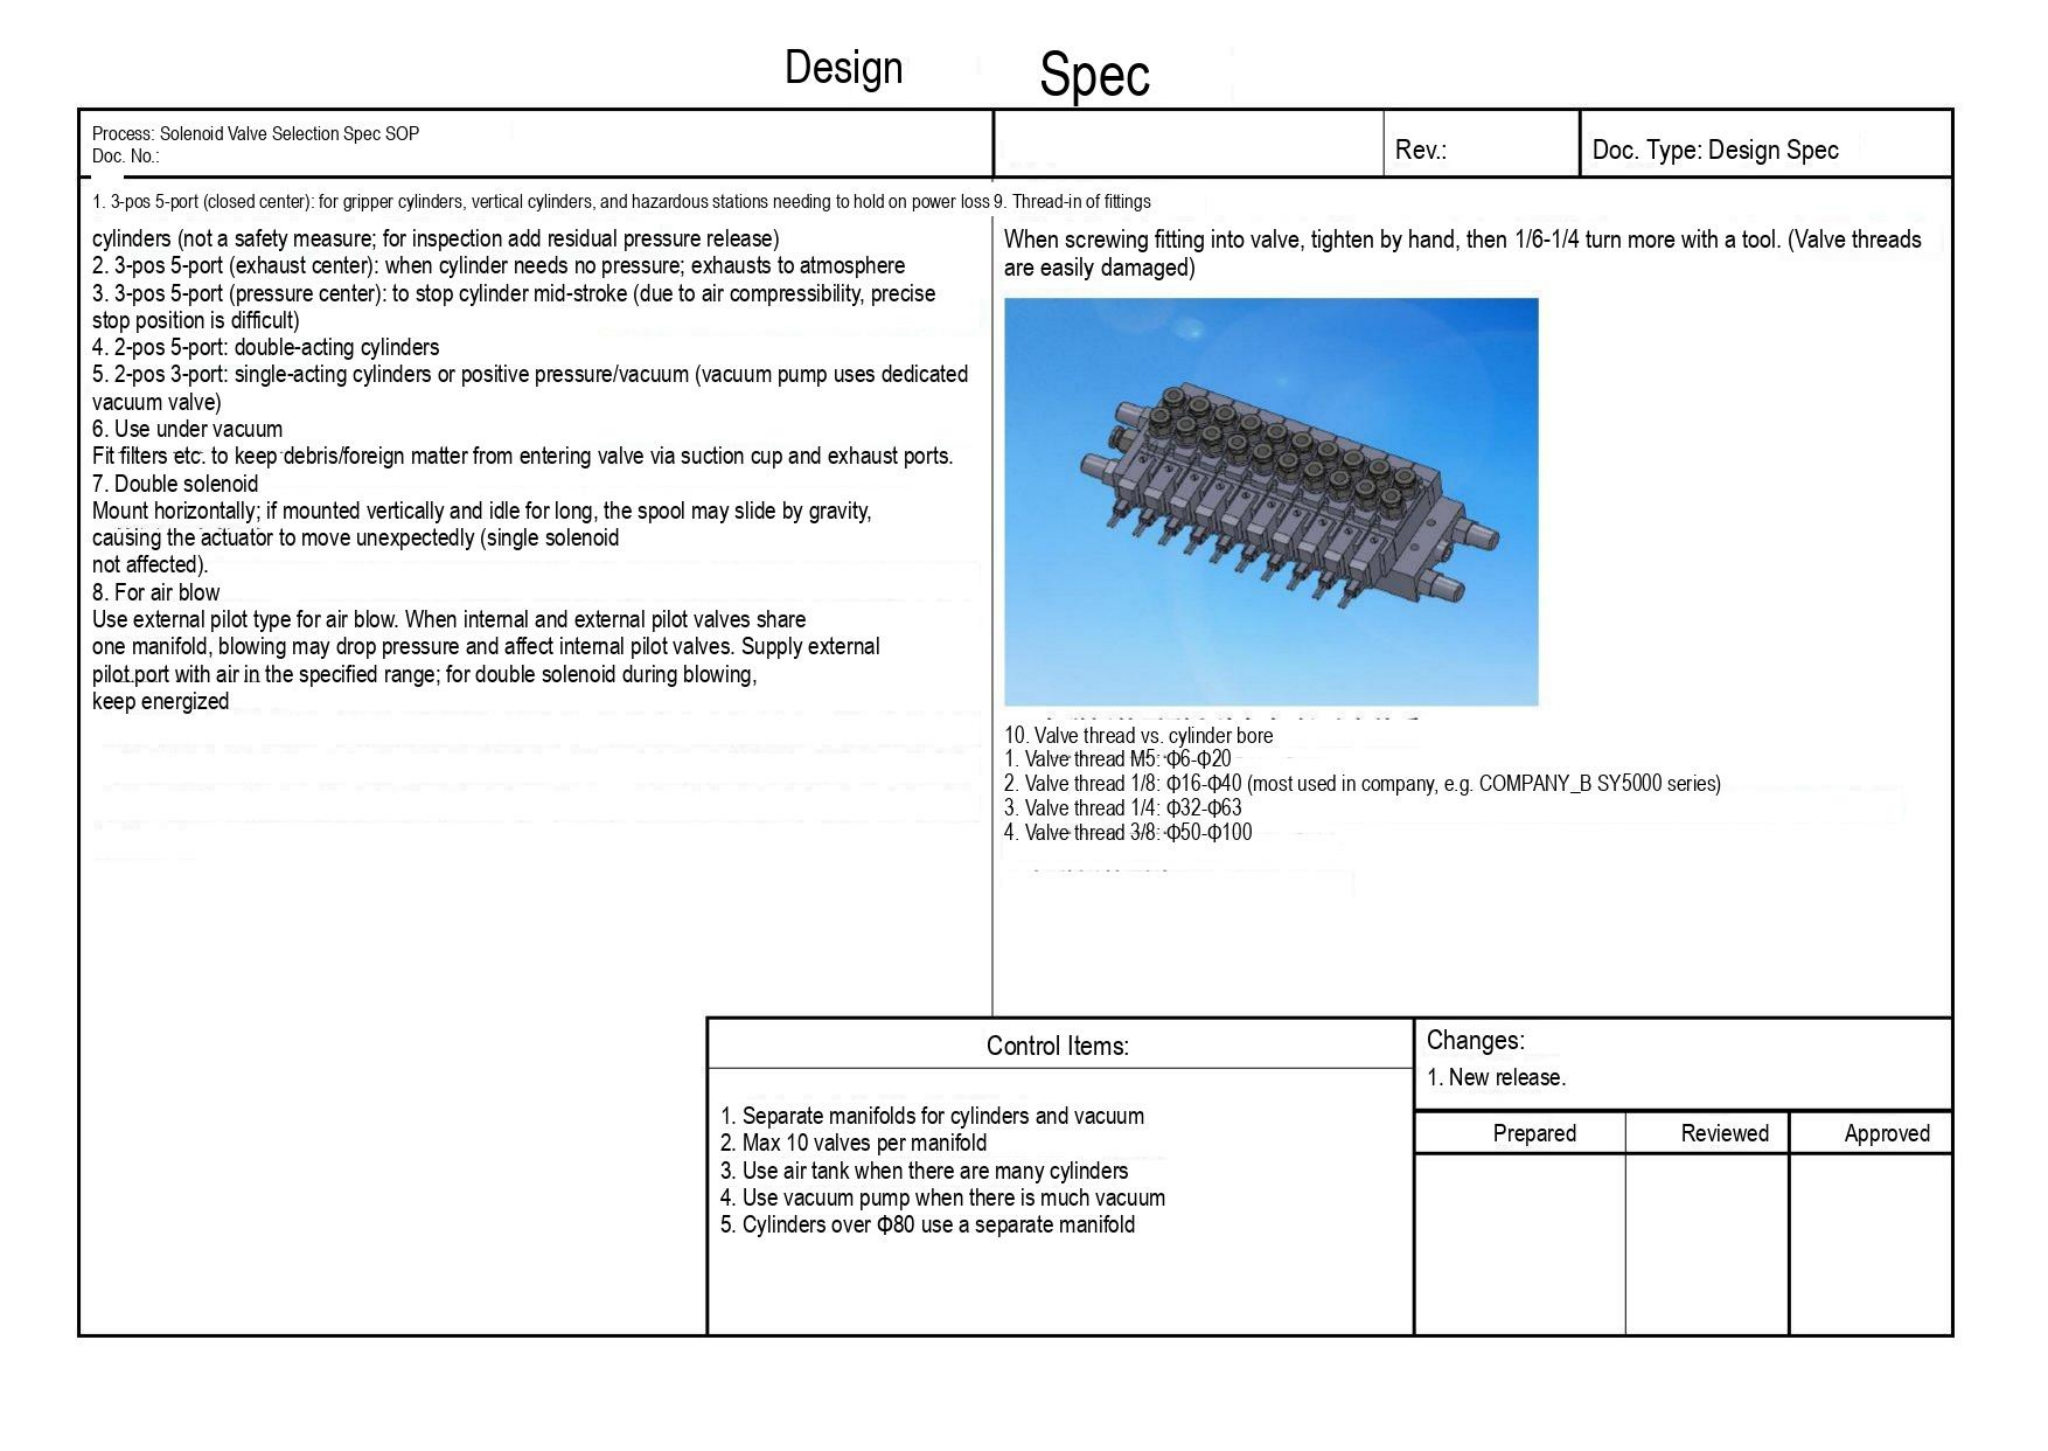Design Spec

| Process: Solenoid Valve Selection Spec SOP<br>Doc. No.: | | Rev.: | Doc. Type: Design Spec |
|---|---|---|---|

1. 3-pos 5-port (closed center): for gripper cylinders, vertical cylinders, and hazardous stations needing to hold on power loss cylinders (not a safety measure; for inspection add residual pressure release)
2. 3-pos 5-port (exhaust center): when cylinder needs no pressure; exhausts to atmosphere
3. 3-pos 5-port (pressure center): to stop cylinder mid-stroke (due to air compressibility, precise stop position is difficult)
4. 2-pos 5-port: double-acting cylinders
5. 2-pos 3-port: single-acting cylinders or positive pressure/vacuum (vacuum pump uses dedicated vacuum valve)
6. Use under vacuum
Fit filters etc. to keep debris/foreign matter from entering valve via suction cup and exhaust ports.
7. Double solenoid
Mount horizontally; if mounted vertically and idle for long, the spool may slide by gravity, causing the actuator to move unexpectedly (single solenoid not affected).
8. For air blow
Use external pilot type for air blow. When internal and external pilot valves share one manifold, blowing may drop pressure and affect internal pilot valves. Supply external pilot port with air in the specified range; for double solenoid during blowing, keep energized

9. Thread-in of fittings
When screwing fitting into valve, tighten by hand, then 1/6-1/4 turn more with a tool. (Valve threads are easily damaged)

10. Valve thread vs. cylinder bore
1. Valve thread M5: Φ6-Φ20
2. Valve thread 1/8: Φ16-Φ40 (most used in company, e.g. COMPANY_B SY5000 series)
3. Valve thread 1/4: Φ32-Φ63
4. Valve thread 3/8: Φ50-Φ100

| Control Items: | Changes: |
|---|---|
| 1. Separate manifolds for cylinders and vacuum<br>2. Max 10 valves per manifold<br>3. Use air tank when there are many cylinders<br>4. Use vacuum pump when there is much vacuum<br>5. Cylinders over Φ80 use a separate manifold | 1. New release. |

| Prepared | Reviewed | Approved |
|---|---|---|
| | | |